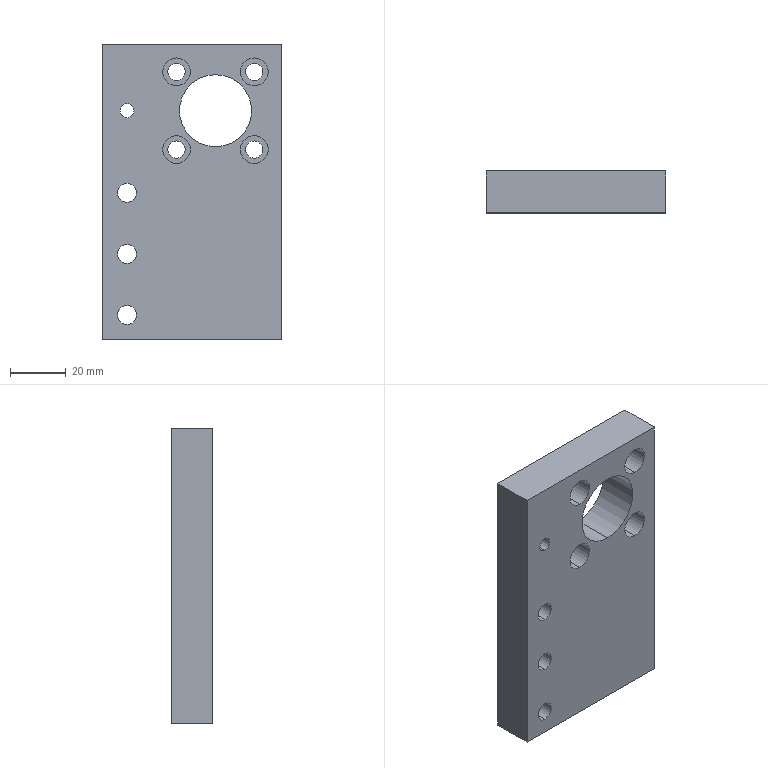Part | 1 solid | 45 faces | box 64.85 x 15 x 106.59 mm | volume 89025 mm3 | cylinder 32 | plane 13 | commonest cylinder face diameters 6.2 x8 10 x8 6.8 x6 11 x6 5 x2 26 x2
STEP:
#1=CARTESIAN_POINT('',(-23.425,0.,26.795));
#2=VERTEX_POINT('',#1);
#3=CARTESIAN_POINT('',(-23.425,0.,31.795));
#4=VERTEX_POINT('',#3);
#5=CARTESIAN_POINT('',(-23.425,0.,29.295));
#6=DIRECTION('',(0.,1.,0.));
#7=DIRECTION('',(0.,0.,1.));
#8=AXIS2_PLACEMENT_3D('',#5,#6,#7);
#9=CIRCLE('',#8,2.5);
#10=EDGE_CURVE('',#2,#4,#9,.T.);
#11=ORIENTED_EDGE('',*,*,#10,.F.);
#12=CARTESIAN_POINT('',(-23.425,15.,26.795));
#13=VERTEX_POINT('',#12);
#14=CARTESIAN_POINT('',(-23.425,15.,26.795));
#15=DIRECTION('',(0.,1.,0.));
#16=VECTOR('',#15,1000.);
#17=LINE('',#14,#16);
#18=EDGE_CURVE('',#2,#13,#17,.T.);
#19=ORIENTED_EDGE('',*,*,#18,.T.);
#20=CARTESIAN_POINT('',(-23.425,15.,31.795));
#21=VERTEX_POINT('',#20);
#22=CARTESIAN_POINT('',(-23.425,15.,29.295));
#23=DIRECTION('',(0.,1.,0.));
#24=DIRECTION('',(0.,0.,1.));
#25=AXIS2_PLACEMENT_3D('',#22,#23,#24);
#26=CIRCLE('',#25,2.5);
#27=EDGE_CURVE('',#13,#21,#26,.T.);
#28=ORIENTED_EDGE('',*,*,#27,.T.);
#29=CARTESIAN_POINT('',(-23.425,15.,31.795));
#30=DIRECTION('',(0.,1.,0.));
#31=VECTOR('',#30,1000.);
#32=LINE('',#29,#31);
#33=EDGE_CURVE('',#4,#21,#32,.T.);
#34=ORIENTED_EDGE('',*,*,#33,.F.);
#35=EDGE_LOOP('',(#11,#19,#28,#34));
#36=FACE_OUTER_BOUND('',#35,.T.);
#37=CARTESIAN_POINT('',(-23.425,15.,29.295));
#38=DIRECTION('',(0.,1.,0.));
#39=DIRECTION('',(0.,0.,1.));
#40=AXIS2_PLACEMENT_3D('',#37,#38,#39);
#41=CYLINDRICAL_SURFACE('',#40,2.5);
#42=ADVANCED_FACE('',(#36),#41,.F.);
#43=CARTESIAN_POINT('',(22.425,8.,48.295));
#44=VERTEX_POINT('',#43);
#45=CARTESIAN_POINT('',(22.425,8.,38.295));
#46=VERTEX_POINT('',#45);
#47=CARTESIAN_POINT('',(22.425,8.,43.295));
#48=DIRECTION('',(0.,-1.,0.));
#49=DIRECTION('',(0.,0.,-1.));
#50=AXIS2_PLACEMENT_3D('',#47,#48,#49);
#51=CIRCLE('',#50,5.);
#52=EDGE_CURVE('',#44,#46,#51,.T.);
#53=ORIENTED_EDGE('',*,*,#52,.F.);
#54=CARTESIAN_POINT('',(22.425,0.,48.295));
#55=VERTEX_POINT('',#54);
#56=CARTESIAN_POINT('',(22.425,8.,48.295));
#57=DIRECTION('',(0.,-1.,0.));
#58=VECTOR('',#57,1000.);
#59=LINE('',#56,#58);
#60=EDGE_CURVE('',#44,#55,#59,.T.);
#61=ORIENTED_EDGE('',*,*,#60,.T.);
#62=CARTESIAN_POINT('',(22.425,0.,38.295));
#63=VERTEX_POINT('',#62);
#64=CARTESIAN_POINT('',(22.425,0.,43.295));
#65=DIRECTION('',(0.,-1.,0.));
#66=DIRECTION('',(0.,0.,-1.));
#67=AXIS2_PLACEMENT_3D('',#64,#65,#66);
#68=CIRCLE('',#67,5.);
#69=EDGE_CURVE('',#55,#63,#68,.T.);
#70=ORIENTED_EDGE('',*,*,#69,.T.);
#71=CARTESIAN_POINT('',(22.425,8.,38.295));
#72=DIRECTION('',(0.,-1.,0.));
#73=VECTOR('',#72,1000.);
#74=LINE('',#71,#73);
#75=EDGE_CURVE('',#46,#63,#74,.T.);
#76=ORIENTED_EDGE('',*,*,#75,.F.);
#77=EDGE_LOOP('',(#53,#61,#70,#76));
#78=FACE_OUTER_BOUND('',#77,.T.);
#79=CARTESIAN_POINT('',(22.425,8.,43.295));
#80=DIRECTION('',(0.,-1.,0.));
#81=DIRECTION('',(0.,0.,-1.));
#82=AXIS2_PLACEMENT_3D('',#79,#80,#81);
#83=CYLINDRICAL_SURFACE('',#82,5.);
#84=ADVANCED_FACE('',(#78),#83,.F.);
#85=CARTESIAN_POINT('',(-5.575,8.,48.295));
#86=VERTEX_POINT('',#85);
#87=CARTESIAN_POINT('',(-5.575,8.,38.295));
#88=VERTEX_POINT('',#87);
#89=CARTESIAN_POINT('',(-5.575,8.,43.295));
#90=DIRECTION('',(0.,-1.,0.));
#91=DIRECTION('',(0.,0.,-1.));
#92=AXIS2_PLACEMENT_3D('',#89,#90,#91);
#93=CIRCLE('',#92,5.);
#94=EDGE_CURVE('',#86,#88,#93,.T.);
#95=ORIENTED_EDGE('',*,*,#94,.F.);
#96=CARTESIAN_POINT('',(-5.575,0.,48.295));
#97=VERTEX_POINT('',#96);
#98=CARTESIAN_POINT('',(-5.575,8.,48.295));
#99=DIRECTION('',(0.,-1.,0.));
#100=VECTOR('',#99,1000.);
#101=LINE('',#98,#100);
#102=EDGE_CURVE('',#86,#97,#101,.T.);
#103=ORIENTED_EDGE('',*,*,#102,.T.);
#104=CARTESIAN_POINT('',(-5.575,0.,38.295));
#105=VERTEX_POINT('',#104);
#106=CARTESIAN_POINT('',(-5.575,0.,43.295));
#107=DIRECTION('',(0.,-1.,0.));
#108=DIRECTION('',(0.,0.,-1.));
#109=AXIS2_PLACEMENT_3D('',#106,#107,#108);
#110=CIRCLE('',#109,5.);
#111=EDGE_CURVE('',#97,#105,#110,.T.);
#112=ORIENTED_EDGE('',*,*,#111,.T.);
#113=CARTESIAN_POINT('',(-5.575,8.,38.295));
#114=DIRECTION('',(0.,-1.,0.));
#115=VECTOR('',#114,1000.);
#116=LINE('',#113,#115);
#117=EDGE_CURVE('',#88,#105,#116,.T.);
#118=ORIENTED_EDGE('',*,*,#117,.F.);
#119=EDGE_LOOP('',(#95,#103,#112,#118));
#120=FACE_OUTER_BOUND('',#119,.T.);
#121=CARTESIAN_POINT('',(-5.575,8.,43.295));
#122=DIRECTION('',(0.,-1.,0.));
#123=DIRECTION('',(0.,0.,-1.));
#124=AXIS2_PLACEMENT_3D('',#121,#122,#123);
#125=CYLINDRICAL_SURFACE('',#124,5.);
#126=ADVANCED_FACE('',(#120),#125,.F.);
#127=CARTESIAN_POINT('',(-5.575,8.,20.295));
#128=VERTEX_POINT('',#127);
#129=CARTESIAN_POINT('',(-5.575,8.,10.295));
#130=VERTEX_POINT('',#129);
#131=CARTESIAN_POINT('',(-5.575,8.,15.295));
#132=DIRECTION('',(0.,-1.,0.));
#133=DIRECTION('',(0.,0.,-1.));
#134=AXIS2_PLACEMENT_3D('',#131,#132,#133);
#135=CIRCLE('',#134,5.);
#136=EDGE_CURVE('',#128,#130,#135,.T.);
#137=ORIENTED_EDGE('',*,*,#136,.F.);
#138=CARTESIAN_POINT('',(-5.575,0.,20.295));
#139=VERTEX_POINT('',#138);
#140=CARTESIAN_POINT('',(-5.575,8.,20.295));
#141=DIRECTION('',(0.,-1.,0.));
#142=VECTOR('',#141,1000.);
#143=LINE('',#140,#142);
#144=EDGE_CURVE('',#128,#139,#143,.T.);
#145=ORIENTED_EDGE('',*,*,#144,.T.);
#146=CARTESIAN_POINT('',(-5.575,0.,10.295));
#147=VERTEX_POINT('',#146);
#148=CARTESIAN_POINT('',(-5.575,0.,15.295));
#149=DIRECTION('',(0.,-1.,0.));
#150=DIRECTION('',(0.,0.,-1.));
#151=AXIS2_PLACEMENT_3D('',#148,#149,#150);
#152=CIRCLE('',#151,5.);
#153=EDGE_CURVE('',#139,#147,#152,.T.);
#154=ORIENTED_EDGE('',*,*,#153,.T.);
#155=CARTESIAN_POINT('',(-5.575,8.,10.295));
#156=DIRECTION('',(0.,-1.,0.));
#157=VECTOR('',#156,1000.);
#158=LINE('',#155,#157);
#159=EDGE_CURVE('',#130,#147,#158,.T.);
#160=ORIENTED_EDGE('',*,*,#159,.F.);
#161=EDGE_LOOP('',(#137,#145,#154,#160));
#162=FACE_OUTER_BOUND('',#161,.T.);
#163=CARTESIAN_POINT('',(-5.575,8.,15.295));
#164=DIRECTION('',(0.,-1.,0.));
#165=DIRECTION('',(0.,0.,-1.));
#166=AXIS2_PLACEMENT_3D('',#163,#164,#165);
#167=CYLINDRICAL_SURFACE('',#166,5.);
#168=ADVANCED_FACE('',(#162),#167,.F.);
#169=CARTESIAN_POINT('',(22.425,8.,20.295));
#170=VERTEX_POINT('',#169);
#171=CARTESIAN_POINT('',(22.425,8.,10.295));
#172=VERTEX_POINT('',#171);
#173=CARTESIAN_POINT('',(22.425,8.,15.295));
#174=DIRECTION('',(0.,-1.,0.));
#175=DIRECTION('',(0.,0.,-1.));
#176=AXIS2_PLACEMENT_3D('',#173,#174,#175);
#177=CIRCLE('',#176,5.);
#178=EDGE_CURVE('',#170,#172,#177,.T.);
#179=ORIENTED_EDGE('',*,*,#178,.F.);
#180=CARTESIAN_POINT('',(22.425,0.,20.295));
#181=VERTEX_POINT('',#180);
#182=CARTESIAN_POINT('',(22.425,8.,20.295));
#183=DIRECTION('',(0.,-1.,0.));
#184=VECTOR('',#183,1000.);
#185=LINE('',#182,#184);
#186=EDGE_CURVE('',#170,#181,#185,.T.);
#187=ORIENTED_EDGE('',*,*,#186,.T.);
#188=CARTESIAN_POINT('',(22.425,0.,10.295));
#189=VERTEX_POINT('',#188);
#190=CARTESIAN_POINT('',(22.425,0.,15.295));
#191=DIRECTION('',(0.,-1.,0.));
#192=DIRECTION('',(0.,0.,-1.));
#193=AXIS2_PLACEMENT_3D('',#190,#191,#192);
#194=CIRCLE('',#193,5.);
#195=EDGE_CURVE('',#181,#189,#194,.T.);
#196=ORIENTED_EDGE('',*,*,#195,.T.);
#197=CARTESIAN_POINT('',(22.425,8.,10.295));
#198=DIRECTION('',(0.,-1.,0.));
#199=VECTOR('',#198,1000.);
#200=LINE('',#197,#199);
#201=EDGE_CURVE('',#172,#189,#200,.T.);
#202=ORIENTED_EDGE('',*,*,#201,.F.);
#203=EDGE_LOOP('',(#179,#187,#196,#202));
#204=FACE_OUTER_BOUND('',#203,.T.);
#205=CARTESIAN_POINT('',(22.425,8.,15.295));
#206=DIRECTION('',(0.,-1.,0.));
#207=DIRECTION('',(0.,0.,-1.));
#208=AXIS2_PLACEMENT_3D('',#205,#206,#207);
#209=CYLINDRICAL_SURFACE('',#208,5.);
#210=ADVANCED_FACE('',(#204),#209,.F.);
#211=CARTESIAN_POINT('',(8.475,0.,16.295));
#212=VERTEX_POINT('',#211);
#213=CARTESIAN_POINT('',(8.475,0.,42.295));
#214=VERTEX_POINT('',#213);
#215=CARTESIAN_POINT('',(8.475,0.,29.295));
#216=DIRECTION('',(0.,1.,0.));
#217=DIRECTION('',(0.,0.,1.));
#218=AXIS2_PLACEMENT_3D('',#215,#216,#217);
#219=CIRCLE('',#218,13.);
#220=EDGE_CURVE('',#212,#214,#219,.T.);
#221=ORIENTED_EDGE('',*,*,#220,.F.);
#222=CARTESIAN_POINT('',(8.475,15.,16.295));
#223=VERTEX_POINT('',#222);
#224=CARTESIAN_POINT('',(8.475,0.,16.295));
#225=DIRECTION('',(0.,1.,0.));
#226=VECTOR('',#225,1000.);
#227=LINE('',#224,#226);
#228=EDGE_CURVE('',#212,#223,#227,.T.);
#229=ORIENTED_EDGE('',*,*,#228,.T.);
#230=CARTESIAN_POINT('',(8.475,15.,42.295));
#231=VERTEX_POINT('',#230);
#232=CARTESIAN_POINT('',(8.475,15.,29.295));
#233=DIRECTION('',(0.,1.,0.));
#234=DIRECTION('',(0.,0.,1.));
#235=AXIS2_PLACEMENT_3D('',#232,#233,#234);
#236=CIRCLE('',#235,13.);
#237=EDGE_CURVE('',#223,#231,#236,.T.);
#238=ORIENTED_EDGE('',*,*,#237,.T.);
#239=CARTESIAN_POINT('',(8.475,0.,42.295));
#240=DIRECTION('',(0.,1.,0.));
#241=VECTOR('',#240,1000.);
#242=LINE('',#239,#241);
#243=EDGE_CURVE('',#214,#231,#242,.T.);
#244=ORIENTED_EDGE('',*,*,#243,.F.);
#245=EDGE_LOOP('',(#221,#229,#238,#244));
#246=FACE_OUTER_BOUND('',#245,.T.);
#247=CARTESIAN_POINT('',(8.475,0.,29.295));
#248=DIRECTION('',(0.,1.,0.));
#249=DIRECTION('',(0.,0.,1.));
#250=AXIS2_PLACEMENT_3D('',#247,#248,#249);
#251=CYLINDRICAL_SURFACE('',#250,13.);
#252=ADVANCED_FACE('',(#246),#251,.F.);
#253=CARTESIAN_POINT('',(-23.425,7.,-5.795));
#254=VERTEX_POINT('',#253);
#255=CARTESIAN_POINT('',(-23.425,7.,5.205));
#256=VERTEX_POINT('',#255);
#257=CARTESIAN_POINT('',(-23.425,7.,-0.295));
#258=DIRECTION('',(0.,1.,0.));
#259=DIRECTION('',(0.,0.,1.));
#260=AXIS2_PLACEMENT_3D('',#257,#258,#259);
#261=CIRCLE('',#260,5.5);
#262=EDGE_CURVE('',#254,#256,#261,.T.);
#263=ORIENTED_EDGE('',*,*,#262,.F.);
#264=CARTESIAN_POINT('',(-23.425,15.,-5.795));
#265=VERTEX_POINT('',#264);
#266=CARTESIAN_POINT('',(-23.425,7.,-5.795));
#267=DIRECTION('',(0.,1.,0.));
#268=VECTOR('',#267,1000.);
#269=LINE('',#266,#268);
#270=EDGE_CURVE('',#254,#265,#269,.T.);
#271=ORIENTED_EDGE('',*,*,#270,.T.);
#272=CARTESIAN_POINT('',(-23.425,15.,5.205));
#273=VERTEX_POINT('',#272);
#274=CARTESIAN_POINT('',(-23.425,15.,-0.295));
#275=DIRECTION('',(0.,1.,0.));
#276=DIRECTION('',(0.,0.,1.));
#277=AXIS2_PLACEMENT_3D('',#274,#275,#276);
#278=CIRCLE('',#277,5.5);
#279=EDGE_CURVE('',#265,#273,#278,.T.);
#280=ORIENTED_EDGE('',*,*,#279,.T.);
#281=CARTESIAN_POINT('',(-23.425,7.,5.205));
#282=DIRECTION('',(0.,1.,0.));
#283=VECTOR('',#282,1000.);
#284=LINE('',#281,#283);
#285=EDGE_CURVE('',#256,#273,#284,.T.);
#286=ORIENTED_EDGE('',*,*,#285,.F.);
#287=EDGE_LOOP('',(#263,#271,#280,#286));
#288=FACE_OUTER_BOUND('',#287,.T.);
#289=CARTESIAN_POINT('',(-23.425,7.,-0.295));
#290=DIRECTION('',(0.,1.,0.));
#291=DIRECTION('',(0.,0.,1.));
#292=AXIS2_PLACEMENT_3D('',#289,#290,#291);
#293=CYLINDRICAL_SURFACE('',#292,5.5);
#294=ADVANCED_FACE('',(#288),#293,.F.);
#295=CARTESIAN_POINT('',(-23.425,7.,-27.795));
#296=VERTEX_POINT('',#295);
#297=CARTESIAN_POINT('',(-23.425,7.,-16.795));
#298=VERTEX_POINT('',#297);
#299=CARTESIAN_POINT('',(-23.425,7.,-22.295));
#300=DIRECTION('',(0.,1.,0.));
#301=DIRECTION('',(0.,0.,1.));
#302=AXIS2_PLACEMENT_3D('',#299,#300,#301);
#303=CIRCLE('',#302,5.5);
#304=EDGE_CURVE('',#296,#298,#303,.T.);
#305=ORIENTED_EDGE('',*,*,#304,.F.);
#306=CARTESIAN_POINT('',(-23.425,15.,-27.795));
#307=VERTEX_POINT('',#306);
#308=CARTESIAN_POINT('',(-23.425,7.,-27.795));
#309=DIRECTION('',(0.,1.,0.));
#310=VECTOR('',#309,1000.);
#311=LINE('',#308,#310);
#312=EDGE_CURVE('',#296,#307,#311,.T.);
#313=ORIENTED_EDGE('',*,*,#312,.T.);
#314=CARTESIAN_POINT('',(-23.425,15.,-16.795));
#315=VERTEX_POINT('',#314);
#316=CARTESIAN_POINT('',(-23.425,15.,-22.295));
#317=DIRECTION('',(0.,1.,0.));
#318=DIRECTION('',(0.,0.,1.));
#319=AXIS2_PLACEMENT_3D('',#316,#317,#318);
#320=CIRCLE('',#319,5.5);
#321=EDGE_CURVE('',#307,#315,#320,.T.);
#322=ORIENTED_EDGE('',*,*,#321,.T.);
#323=CARTESIAN_POINT('',(-23.425,7.,-16.795));
#324=DIRECTION('',(0.,1.,0.));
#325=VECTOR('',#324,1000.);
#326=LINE('',#323,#325);
#327=EDGE_CURVE('',#298,#315,#326,.T.);
#328=ORIENTED_EDGE('',*,*,#327,.F.);
#329=EDGE_LOOP('',(#305,#313,#322,#328));
#330=FACE_OUTER_BOUND('',#329,.T.);
#331=CARTESIAN_POINT('',(-23.425,7.,-22.295));
#332=DIRECTION('',(0.,1.,0.));
#333=DIRECTION('',(0.,0.,1.));
#334=AXIS2_PLACEMENT_3D('',#331,#332,#333);
#335=CYLINDRICAL_SURFACE('',#334,5.5);
#336=ADVANCED_FACE('',(#330),#335,.F.);
#337=CARTESIAN_POINT('',(-23.425,7.,-49.795));
#338=VERTEX_POINT('',#337);
#339=CARTESIAN_POINT('',(-23.425,7.,-38.795));
#340=VERTEX_POINT('',#339);
#341=CARTESIAN_POINT('',(-23.425,7.,-44.295));
#342=DIRECTION('',(0.,1.,0.));
#343=DIRECTION('',(0.,0.,1.));
#344=AXIS2_PLACEMENT_3D('',#341,#342,#343);
#345=CIRCLE('',#344,5.5);
#346=EDGE_CURVE('',#338,#340,#345,.T.);
#347=ORIENTED_EDGE('',*,*,#346,.F.);
#348=CARTESIAN_POINT('',(-23.425,15.,-49.795));
#349=VERTEX_POINT('',#348);
#350=CARTESIAN_POINT('',(-23.425,7.,-49.795));
#351=DIRECTION('',(0.,1.,0.));
#352=VECTOR('',#351,1000.);
#353=LINE('',#350,#352);
#354=EDGE_CURVE('',#338,#349,#353,.T.);
#355=ORIENTED_EDGE('',*,*,#354,.T.);
#356=CARTESIAN_POINT('',(-23.425,15.,-38.795));
#357=VERTEX_POINT('',#356);
#358=CARTESIAN_POINT('',(-23.425,15.,-44.295));
#359=DIRECTION('',(0.,1.,0.));
#360=DIRECTION('',(0.,0.,1.));
#361=AXIS2_PLACEMENT_3D('',#358,#359,#360);
#362=CIRCLE('',#361,5.5);
#363=EDGE_CURVE('',#349,#357,#362,.T.);
#364=ORIENTED_EDGE('',*,*,#363,.T.);
#365=CARTESIAN_POINT('',(-23.425,7.,-38.795));
#366=DIRECTION('',(0.,1.,0.));
#367=VECTOR('',#366,1000.);
#368=LINE('',#365,#367);
#369=EDGE_CURVE('',#340,#357,#368,.T.);
#370=ORIENTED_EDGE('',*,*,#369,.F.);
#371=EDGE_LOOP('',(#347,#355,#364,#370));
#372=FACE_OUTER_BOUND('',#371,.T.);
#373=CARTESIAN_POINT('',(-23.425,7.,-44.295));
#374=DIRECTION('',(0.,1.,0.));
#375=DIRECTION('',(0.,0.,1.));
#376=AXIS2_PLACEMENT_3D('',#373,#374,#375);
#377=CYLINDRICAL_SURFACE('',#376,5.5);
#378=ADVANCED_FACE('',(#372),#377,.F.);
#379=CARTESIAN_POINT('',(-23.425,0.,-47.695));
#380=VERTEX_POINT('',#379);
#381=CARTESIAN_POINT('',(-23.425,0.,-40.895));
#382=VERTEX_POINT('',#381);
#383=CARTESIAN_POINT('',(-23.425,0.,-44.295));
#384=DIRECTION('',(0.,1.,0.));
#385=DIRECTION('',(0.,0.,1.));
#386=AXIS2_PLACEMENT_3D('',#383,#384,#385);
#387=CIRCLE('',#386,3.4);
#388=EDGE_CURVE('',#380,#382,#387,.T.);
#389=ORIENTED_EDGE('',*,*,#388,.F.);
#390=CARTESIAN_POINT('',(-23.425,7.,-47.695));
#391=VERTEX_POINT('',#390);
#392=CARTESIAN_POINT('',(-23.425,0.,-47.695));
#393=DIRECTION('',(0.,1.,0.));
#394=VECTOR('',#393,1000.);
#395=LINE('',#392,#394);
#396=EDGE_CURVE('',#380,#391,#395,.T.);
#397=ORIENTED_EDGE('',*,*,#396,.T.);
#398=CARTESIAN_POINT('',(-23.425,7.,-40.895));
#399=VERTEX_POINT('',#398);
#400=CARTESIAN_POINT('',(-23.425,7.,-44.295));
#401=DIRECTION('',(0.,-1.,0.));
#402=DIRECTION('',(0.,0.,1.));
#403=AXIS2_PLACEMENT_3D('',#400,#401,#402);
#404=CIRCLE('',#403,3.4);
#405=EDGE_CURVE('',#399,#391,#404,.T.);
#406=ORIENTED_EDGE('',*,*,#405,.F.);
#407=CARTESIAN_POINT('',(-23.425,0.,-40.895));
#408=DIRECTION('',(0.,1.,0.));
#409=VECTOR('',#408,1000.);
#410=LINE('',#407,#409);
#411=EDGE_CURVE('',#382,#399,#410,.T.);
#412=ORIENTED_EDGE('',*,*,#411,.F.);
#413=EDGE_LOOP('',(#389,#397,#406,#412));
#414=FACE_OUTER_BOUND('',#413,.T.);
#415=CARTESIAN_POINT('',(-23.425,0.,-44.295));
#416=DIRECTION('',(0.,1.,0.));
#417=DIRECTION('',(0.,0.,1.));
#418=AXIS2_PLACEMENT_3D('',#415,#416,#417);
#419=CYLINDRICAL_SURFACE('',#418,3.4);
#420=ADVANCED_FACE('',(#414),#419,.F.);
#421=CARTESIAN_POINT('',(-23.425,0.,-25.695));
#422=VERTEX_POINT('',#421);
#423=CARTESIAN_POINT('',(-23.425,0.,-18.895));
#424=VERTEX_POINT('',#423);
#425=CARTESIAN_POINT('',(-23.425,0.,-22.295));
#426=DIRECTION('',(0.,1.,0.));
#427=DIRECTION('',(0.,0.,1.));
#428=AXIS2_PLACEMENT_3D('',#425,#426,#427);
#429=CIRCLE('',#428,3.4);
#430=EDGE_CURVE('',#422,#424,#429,.T.);
#431=ORIENTED_EDGE('',*,*,#430,.F.);
#432=CARTESIAN_POINT('',(-23.425,7.,-25.695));
#433=VERTEX_POINT('',#432);
#434=CARTESIAN_POINT('',(-23.425,0.,-25.695));
#435=DIRECTION('',(0.,1.,0.));
#436=VECTOR('',#435,1000.);
#437=LINE('',#434,#436);
#438=EDGE_CURVE('',#422,#433,#437,.T.);
#439=ORIENTED_EDGE('',*,*,#438,.T.);
#440=CARTESIAN_POINT('',(-23.425,7.,-18.895));
#441=VERTEX_POINT('',#440);
#442=CARTESIAN_POINT('',(-23.425,7.,-22.295));
#443=DIRECTION('',(0.,-1.,0.));
#444=DIRECTION('',(0.,0.,1.));
#445=AXIS2_PLACEMENT_3D('',#442,#443,#444);
#446=CIRCLE('',#445,3.4);
#447=EDGE_CURVE('',#441,#433,#446,.T.);
#448=ORIENTED_EDGE('',*,*,#447,.F.);
#449=CARTESIAN_POINT('',(-23.425,0.,-18.895));
#450=DIRECTION('',(0.,1.,0.));
#451=VECTOR('',#450,1000.);
#452=LINE('',#449,#451);
#453=EDGE_CURVE('',#424,#441,#452,.T.);
#454=ORIENTED_EDGE('',*,*,#453,.F.);
#455=EDGE_LOOP('',(#431,#439,#448,#454));
#456=FACE_OUTER_BOUND('',#455,.T.);
#457=CARTESIAN_POINT('',(-23.425,0.,-22.295));
#458=DIRECTION('',(0.,1.,0.));
#459=DIRECTION('',(0.,0.,1.));
#460=AXIS2_PLACEMENT_3D('',#457,#458,#459);
#461=CYLINDRICAL_SURFACE('',#460,3.4);
#462=ADVANCED_FACE('',(#456),#461,.F.);
#463=CARTESIAN_POINT('',(-23.425,0.,-3.695));
#464=VERTEX_POINT('',#463);
#465=CARTESIAN_POINT('',(-23.425,0.,3.105));
#466=VERTEX_POINT('',#465);
#467=CARTESIAN_POINT('',(-23.425,0.,-0.295));
#468=DIRECTION('',(0.,1.,0.));
#469=DIRECTION('',(0.,0.,1.));
#470=AXIS2_PLACEMENT_3D('',#467,#468,#469);
#471=CIRCLE('',#470,3.4);
#472=EDGE_CURVE('',#464,#466,#471,.T.);
#473=ORIENTED_EDGE('',*,*,#472,.F.);
#474=CARTESIAN_POINT('',(-23.425,7.,-3.695));
#475=VERTEX_POINT('',#474);
#476=CARTESIAN_POINT('',(-23.425,0.,-3.695));
#477=DIRECTION('',(0.,1.,0.));
#478=VECTOR('',#477,1000.);
#479=LINE('',#476,#478);
#480=EDGE_CURVE('',#464,#475,#479,.T.);
#481=ORIENTED_EDGE('',*,*,#480,.T.);
#482=CARTESIAN_POINT('',(-23.425,7.,3.105));
#483=VERTEX_POINT('',#482);
#484=CARTESIAN_POINT('',(-23.425,7.,-0.295));
#485=DIRECTION('',(0.,-1.,0.));
#486=DIRECTION('',(0.,0.,1.));
#487=AXIS2_PLACEMENT_3D('',#484,#485,#486);
#488=CIRCLE('',#487,3.4);
#489=EDGE_CURVE('',#483,#475,#488,.T.);
#490=ORIENTED_EDGE('',*,*,#489,.F.);
#491=CARTESIAN_POINT('',(-23.425,0.,3.105));
#492=DIRECTION('',(0.,1.,0.));
#493=VECTOR('',#492,1000.);
#494=LINE('',#491,#493);
#495=EDGE_CURVE('',#466,#483,#494,.T.);
#496=ORIENTED_EDGE('',*,*,#495,.F.);
#497=EDGE_LOOP('',(#473,#481,#490,#496));
#498=FACE_OUTER_BOUND('',#497,.T.);
#499=CARTESIAN_POINT('',(-23.425,0.,-0.295));
#500=DIRECTION('',(0.,1.,0.));
#501=DIRECTION('',(0.,0.,1.));
#502=AXIS2_PLACEMENT_3D('',#499,#500,#501);
#503=CYLINDRICAL_SURFACE('',#502,3.4);
#504=ADVANCED_FACE('',(#498),#503,.F.);
#505=CARTESIAN_POINT('',(22.425,8.,12.195));
#506=VERTEX_POINT('',#505);
#507=CARTESIAN_POINT('',(22.425,8.,18.395));
#508=VERTEX_POINT('',#507);
#509=CARTESIAN_POINT('',(22.425,8.,15.295));
#510=DIRECTION('',(0.,1.,0.));
#511=DIRECTION('',(0.,0.,-1.));
#512=AXIS2_PLACEMENT_3D('',#509,#510,#511);
#513=CIRCLE('',#512,3.1);
#514=EDGE_CURVE('',#506,#508,#513,.T.);
#515=ORIENTED_EDGE('',*,*,#514,.F.);
#516=CARTESIAN_POINT('',(22.425,15.,12.195));
#517=VERTEX_POINT('',#516);
#518=CARTESIAN_POINT('',(22.425,0.,12.195));
#519=DIRECTION('',(0.,1.,0.));
#520=VECTOR('',#519,1000.);
#521=LINE('',#518,#520);
#522=EDGE_CURVE('',#506,#517,#521,.T.);
#523=ORIENTED_EDGE('',*,*,#522,.T.);
#524=CARTESIAN_POINT('',(22.425,15.,18.395));
#525=VERTEX_POINT('',#524);
#526=CARTESIAN_POINT('',(22.425,15.,15.295));
#527=DIRECTION('',(0.,1.,0.));
#528=DIRECTION('',(0.,0.,1.));
#529=AXIS2_PLACEMENT_3D('',#526,#527,#528);
#530=CIRCLE('',#529,3.1);
#531=EDGE_CURVE('',#517,#525,#530,.T.);
#532=ORIENTED_EDGE('',*,*,#531,.T.);
#533=CARTESIAN_POINT('',(22.425,0.,18.395));
#534=DIRECTION('',(0.,1.,0.));
#535=VECTOR('',#534,1000.);
#536=LINE('',#533,#535);
#537=EDGE_CURVE('',#508,#525,#536,.T.);
#538=ORIENTED_EDGE('',*,*,#537,.F.);
#539=EDGE_LOOP('',(#515,#523,#532,#538));
#540=FACE_OUTER_BOUND('',#539,.T.);
#541=CARTESIAN_POINT('',(22.425,0.,15.295));
#542=DIRECTION('',(0.,1.,0.));
#543=DIRECTION('',(0.,0.,1.));
#544=AXIS2_PLACEMENT_3D('',#541,#542,#543);
#545=CYLINDRICAL_SURFACE('',#544,3.1);
#546=ADVANCED_FACE('',(#540),#545,.F.);
#547=CARTESIAN_POINT('',(-5.575,8.,12.195));
#548=VERTEX_POINT('',#547);
#549=CARTESIAN_POINT('',(-5.575,8.,18.395));
#550=VERTEX_POINT('',#549);
#551=CARTESIAN_POINT('',(-5.575,8.,15.295));
#552=DIRECTION('',(0.,1.,0.));
#553=DIRECTION('',(0.,0.,-1.));
#554=AXIS2_PLACEMENT_3D('',#551,#552,#553);
#555=CIRCLE('',#554,3.1);
#556=EDGE_CURVE('',#548,#550,#555,.T.);
#557=ORIENTED_EDGE('',*,*,#556,.F.);
#558=CARTESIAN_POINT('',(-5.575,15.,12.195));
#559=VERTEX_POINT('',#558);
#560=CARTESIAN_POINT('',(-5.575,0.,12.195));
#561=DIRECTION('',(0.,1.,0.));
#562=VECTOR('',#561,1000.);
#563=LINE('',#560,#562);
#564=EDGE_CURVE('',#548,#559,#563,.T.);
#565=ORIENTED_EDGE('',*,*,#564,.T.);
#566=CARTESIAN_POINT('',(-5.575,15.,18.395));
#567=VERTEX_POINT('',#566);
#568=CARTESIAN_POINT('',(-5.575,15.,15.295));
#569=DIRECTION('',(0.,1.,0.));
#570=DIRECTION('',(0.,0.,1.));
#571=AXIS2_PLACEMENT_3D('',#568,#569,#570);
#572=CIRCLE('',#571,3.1);
#573=EDGE_CURVE('',#559,#567,#572,.T.);
#574=ORIENTED_EDGE('',*,*,#573,.T.);
#575=CARTESIAN_POINT('',(-5.575,0.,18.395));
#576=DIRECTION('',(0.,1.,0.));
#577=VECTOR('',#576,1000.);
#578=LINE('',#575,#577);
#579=EDGE_CURVE('',#550,#567,#578,.T.);
#580=ORIENTED_EDGE('',*,*,#579,.F.);
#581=EDGE_LOOP('',(#557,#565,#574,#580));
#582=FACE_OUTER_BOUND('',#581,.T.);
#583=CARTESIAN_POINT('',(-5.575,0.,15.295));
#584=DIRECTION('',(0.,1.,0.));
#585=DIRECTION('',(0.,0.,1.));
#586=AXIS2_PLACEMENT_3D('',#583,#584,#585);
#587=CYLINDRICAL_SURFACE('',#586,3.1);
#588=ADVANCED_FACE('',(#582),#587,.F.);
#589=CARTESIAN_POINT('',(-5.575,8.,40.195));
#590=VERTEX_POINT('',#589);
#591=CARTESIAN_POINT('',(-5.575,8.,46.395));
#592=VERTEX_POINT('',#591);
#593=CARTESIAN_POINT('',(-5.575,8.,43.295));
#594=DIRECTION('',(0.,1.,0.));
#595=DIRECTION('',(0.,0.,-1.));
#596=AXIS2_PLACEMENT_3D('',#593,#594,#595);
#597=CIRCLE('',#596,3.1);
#598=EDGE_CURVE('',#590,#592,#597,.T.);
#599=ORIENTED_EDGE('',*,*,#598,.F.);
#600=CARTESIAN_POINT('',(-5.575,15.,40.195));
#601=VERTEX_POINT('',#600);
#602=CARTESIAN_POINT('',(-5.575,0.,40.195));
#603=DIRECTION('',(0.,1.,0.));
#604=VECTOR('',#603,1000.);
#605=LINE('',#602,#604);
#606=EDGE_CURVE('',#590,#601,#605,.T.);
#607=ORIENTED_EDGE('',*,*,#606,.T.);
#608=CARTESIAN_POINT('',(-5.575,15.,46.395));
#609=VERTEX_POINT('',#608);
#610=CARTESIAN_POINT('',(-5.575,15.,43.295));
#611=DIRECTION('',(0.,1.,0.));
#612=DIRECTION('',(0.,0.,1.));
#613=AXIS2_PLACEMENT_3D('',#610,#611,#612);
#614=CIRCLE('',#613,3.1);
#615=EDGE_CURVE('',#601,#609,#614,.T.);
#616=ORIENTED_EDGE('',*,*,#615,.T.);
#617=CARTESIAN_POINT('',(-5.575,0.,46.395));
#618=DIRECTION('',(0.,1.,0.));
#619=VECTOR('',#618,1000.);
#620=LINE('',#617,#619);
#621=EDGE_CURVE('',#592,#609,#620,.T.);
#622=ORIENTED_EDGE('',*,*,#621,.F.);
#623=EDGE_LOOP('',(#599,#607,#616,#622));
#624=FACE_OUTER_BOUND('',#623,.T.);
#625=CARTESIAN_POINT('',(-5.575,0.,43.295));
#626=DIRECTION('',(0.,1.,0.));
#627=DIRECTION('',(0.,0.,1.));
#628=AXIS2_PLACEMENT_3D('',#625,#626,#627);
#629=CYLINDRICAL_SURFACE('',#628,3.1);
#630=ADVANCED_FACE('',(#624),#629,.F.);
#631=CARTESIAN_POINT('',(22.425,8.,40.195));
#632=VERTEX_POINT('',#631);
#633=CARTESIAN_POINT('',(22.425,8.,46.395));
#634=VERTEX_POINT('',#633);
#635=CARTESIAN_POINT('',(22.425,8.,43.295));
#636=DIRECTION('',(0.,1.,0.));
#637=DIRECTION('',(0.,0.,-1.));
#638=AXIS2_PLACEMENT_3D('',#635,#636,#637);
#639=CIRCLE('',#638,3.1);
#640=EDGE_CURVE('',#632,#634,#639,.T.);
#641=ORIENTED_EDGE('',*,*,#640,.F.);
#642=CARTESIAN_POINT('',(22.425,15.,40.195));
#643=VERTEX_POINT('',#642);
#644=CARTESIAN_POINT('',(22.425,0.,40.195));
#645=DIRECTION('',(0.,1.,0.));
#646=VECTOR('',#645,1000.);
#647=LINE('',#644,#646);
#648=EDGE_CURVE('',#632,#643,#647,.T.);
#649=ORIENTED_EDGE('',*,*,#648,.T.);
#650=CARTESIAN_POINT('',(22.425,15.,46.395));
#651=VERTEX_POINT('',#650);
#652=CARTESIAN_POINT('',(22.425,15.,43.295));
#653=DIRECTION('',(0.,1.,0.));
#654=DIRECTION('',(0.,0.,1.));
#655=AXIS2_PLACEMENT_3D('',#652,#653,#654);
#656=CIRCLE('',#655,3.1);
#657=EDGE_CURVE('',#643,#651,#656,.T.);
#658=ORIENTED_EDGE('',*,*,#657,.T.);
#659=CARTESIAN_POINT('',(22.425,0.,46.395));
#660=DIRECTION('',(0.,1.,0.));
#661=VECTOR('',#660,1000.);
#662=LINE('',#659,#661);
#663=EDGE_CURVE('',#634,#651,#662,.T.);
#664=ORIENTED_EDGE('',*,*,#663,.F.);
#665=EDGE_LOOP('',(#641,#649,#658,#664));
#666=FACE_OUTER_BOUND('',#665,.T.);
#667=CARTESIAN_POINT('',(22.425,0.,43.295));
#668=DIRECTION('',(0.,1.,0.));
#669=DIRECTION('',(0.,0.,1.));
#670=AXIS2_PLACEMENT_3D('',#667,#668,#669);
#671=CYLINDRICAL_SURFACE('',#670,3.1);
#672=ADVANCED_FACE('',(#666),#671,.F.);
#673=ORIENTED_EDGE('',*,*,#648,.F.);
#674=CARTESIAN_POINT('',(22.425,8.,43.295));
#675=DIRECTION('',(0.,1.,0.));
#676=DIRECTION('',(0.,0.,-1.));
#677=AXIS2_PLACEMENT_3D('',#674,#675,#676);
#678=CIRCLE('',#677,3.1);
#679=EDGE_CURVE('',#634,#632,#678,.T.);
#680=ORIENTED_EDGE('',*,*,#679,.F.);
#681=ORIENTED_EDGE('',*,*,#663,.T.);
#682=CARTESIAN_POINT('',(22.425,15.,43.295));
#683=DIRECTION('',(0.,1.,0.));
#684=DIRECTION('',(0.,0.,1.));
#685=AXIS2_PLACEMENT_3D('',#682,#683,#684);
#686=CIRCLE('',#685,3.1);
#687=EDGE_CURVE('',#651,#643,#686,.T.);
#688=ORIENTED_EDGE('',*,*,#687,.T.);
#689=EDGE_LOOP('',(#673,#680,#681,#688));
#690=FACE_OUTER_BOUND('',#689,.T.);
#691=CARTESIAN_POINT('',(22.425,0.,43.295));
#692=DIRECTION('',(0.,1.,0.));
#693=DIRECTION('',(0.,0.,1.));
#694=AXIS2_PLACEMENT_3D('',#691,#692,#693);
#695=CYLINDRICAL_SURFACE('',#694,3.1);
#696=ADVANCED_FACE('',(#690),#695,.F.);
#697=ORIENTED_EDGE('',*,*,#606,.F.);
#698=CARTESIAN_POINT('',(-5.575,8.,43.295));
#699=DIRECTION('',(0.,1.,0.));
#700=DIRECTION('',(0.,0.,-1.));
#701=AXIS2_PLACEMENT_3D('',#698,#699,#700);
#702=CIRCLE('',#701,3.1);
#703=EDGE_CURVE('',#592,#590,#702,.T.);
#704=ORIENTED_EDGE('',*,*,#703,.F.);
#705=ORIENTED_EDGE('',*,*,#621,.T.);
#706=CARTESIAN_POINT('',(-5.575,15.,43.295));
#707=DIRECTION('',(0.,1.,0.));
#708=DIRECTION('',(0.,0.,1.));
#709=AXIS2_PLACEMENT_3D('',#706,#707,#708);
#710=CIRCLE('',#709,3.1);
#711=EDGE_CURVE('',#609,#601,#710,.T.);
#712=ORIENTED_EDGE('',*,*,#711,.T.);
#713=EDGE_LOOP('',(#697,#704,#705,#712));
#714=FACE_OUTER_BOUND('',#713,.T.);
#715=CARTESIAN_POINT('',(-5.575,0.,43.295));
#716=DIRECTION('',(0.,1.,0.));
#717=DIRECTION('',(0.,0.,1.));
#718=AXIS2_PLACEMENT_3D('',#715,#716,#717);
#719=CYLINDRICAL_SURFACE('',#718,3.1);
#720=ADVANCED_FACE('',(#714),#719,.F.);
#721=ORIENTED_EDGE('',*,*,#564,.F.);
#722=CARTESIAN_POINT('',(-5.575,8.,15.295));
#723=DIRECTION('',(0.,1.,0.));
#724=DIRECTION('',(0.,0.,-1.));
#725=AXIS2_PLACEMENT_3D('',#722,#723,#724);
#726=CIRCLE('',#725,3.1);
#727=EDGE_CURVE('',#550,#548,#726,.T.);
#728=ORIENTED_EDGE('',*,*,#727,.F.);
#729=ORIENTED_EDGE('',*,*,#579,.T.);
#730=CARTESIAN_POINT('',(-5.575,15.,15.295));
#731=DIRECTION('',(0.,1.,0.));
#732=DIRECTION('',(0.,0.,1.));
#733=AXIS2_PLACEMENT_3D('',#730,#731,#732);
#734=CIRCLE('',#733,3.1);
#735=EDGE_CURVE('',#567,#559,#734,.T.);
#736=ORIENTED_EDGE('',*,*,#735,.T.);
#737=EDGE_LOOP('',(#721,#728,#729,#736));
#738=FACE_OUTER_BOUND('',#737,.T.);
#739=CARTESIAN_POINT('',(-5.575,0.,15.295));
#740=DIRECTION('',(0.,1.,0.));
#741=DIRECTION('',(0.,0.,1.));
#742=AXIS2_PLACEMENT_3D('',#739,#740,#741);
#743=CYLINDRICAL_SURFACE('',#742,3.1);
#744=ADVANCED_FACE('',(#738),#743,.F.);
#745=ORIENTED_EDGE('',*,*,#522,.F.);
#746=CARTESIAN_POINT('',(22.425,8.,15.295));
#747=DIRECTION('',(0.,1.,0.));
#748=DIRECTION('',(0.,0.,-1.));
#749=AXIS2_PLACEMENT_3D('',#746,#747,#748);
#750=CIRCLE('',#749,3.1);
#751=EDGE_CURVE('',#508,#506,#750,.T.);
#752=ORIENTED_EDGE('',*,*,#751,.F.);
#753=ORIENTED_EDGE('',*,*,#537,.T.);
#754=CARTESIAN_POINT('',(22.425,15.,15.295));
#755=DIRECTION('',(0.,1.,0.));
#756=DIRECTION('',(0.,0.,1.));
#757=AXIS2_PLACEMENT_3D('',#754,#755,#756);
#758=CIRCLE('',#757,3.1);
#759=EDGE_CURVE('',#525,#517,#758,.T.);
#760=ORIENTED_EDGE('',*,*,#759,.T.);
#761=EDGE_LOOP('',(#745,#752,#753,#760));
#762=FACE_OUTER_BOUND('',#761,.T.);
#763=CARTESIAN_POINT('',(22.425,0.,15.295));
#764=DIRECTION('',(0.,1.,0.));
#765=DIRECTION('',(0.,0.,1.));
#766=AXIS2_PLACEMENT_3D('',#763,#764,#765);
#767=CYLINDRICAL_SURFACE('',#766,3.1);
#768=ADVANCED_FACE('',(#762),#767,.F.);
#769=ORIENTED_EDGE('',*,*,#480,.F.);
#770=CARTESIAN_POINT('',(-23.425,0.,-0.295));
#771=DIRECTION('',(0.,1.,0.));
#772=DIRECTION('',(0.,0.,1.));
#773=AXIS2_PLACEMENT_3D('',#770,#771,#772);
#774=CIRCLE('',#773,3.4);
#775=EDGE_CURVE('',#466,#464,#774,.T.);
#776=ORIENTED_EDGE('',*,*,#775,.F.);
#777=ORIENTED_EDGE('',*,*,#495,.T.);
#778=CARTESIAN_POINT('',(-23.425,7.,-0.295));
#779=DIRECTION('',(0.,-1.,0.));
#780=DIRECTION('',(0.,0.,1.));
#781=AXIS2_PLACEMENT_3D('',#778,#779,#780);
#782=CIRCLE('',#781,3.4);
#783=EDGE_CURVE('',#475,#483,#782,.T.);
#784=ORIENTED_EDGE('',*,*,#783,.F.);
#785=EDGE_LOOP('',(#769,#776,#777,#784));
#786=FACE_OUTER_BOUND('',#785,.T.);
#787=CARTESIAN_POINT('',(-23.425,0.,-0.295));
#788=DIRECTION('',(0.,1.,0.));
#789=DIRECTION('',(0.,0.,1.));
#790=AXIS2_PLACEMENT_3D('',#787,#788,#789);
#791=CYLINDRICAL_SURFACE('',#790,3.4);
#792=ADVANCED_FACE('',(#786),#791,.F.);
#793=ORIENTED_EDGE('',*,*,#438,.F.);
#794=CARTESIAN_POINT('',(-23.425,0.,-22.295));
#795=DIRECTION('',(0.,1.,0.));
#796=DIRECTION('',(0.,0.,1.));
#797=AXIS2_PLACEMENT_3D('',#794,#795,#796);
#798=CIRCLE('',#797,3.4);
#799=EDGE_CURVE('',#424,#422,#798,.T.);
#800=ORIENTED_EDGE('',*,*,#799,.F.);
#801=ORIENTED_EDGE('',*,*,#453,.T.);
#802=CARTESIAN_POINT('',(-23.425,7.,-22.295));
#803=DIRECTION('',(0.,-1.,0.));
#804=DIRECTION('',(0.,0.,1.));
#805=AXIS2_PLACEMENT_3D('',#802,#803,#804);
#806=CIRCLE('',#805,3.4);
#807=EDGE_CURVE('',#433,#441,#806,.T.);
#808=ORIENTED_EDGE('',*,*,#807,.F.);
#809=EDGE_LOOP('',(#793,#800,#801,#808));
#810=FACE_OUTER_BOUND('',#809,.T.);
#811=CARTESIAN_POINT('',(-23.425,0.,-22.295));
#812=DIRECTION('',(0.,1.,0.));
#813=DIRECTION('',(0.,0.,1.));
#814=AXIS2_PLACEMENT_3D('',#811,#812,#813);
#815=CYLINDRICAL_SURFACE('',#814,3.4);
#816=ADVANCED_FACE('',(#810),#815,.F.);
#817=ORIENTED_EDGE('',*,*,#396,.F.);
#818=CARTESIAN_POINT('',(-23.425,0.,-44.295));
#819=DIRECTION('',(0.,1.,0.));
#820=DIRECTION('',(0.,0.,1.));
#821=AXIS2_PLACEMENT_3D('',#818,#819,#820);
#822=CIRCLE('',#821,3.4);
#823=EDGE_CURVE('',#382,#380,#822,.T.);
#824=ORIENTED_EDGE('',*,*,#823,.F.);
#825=ORIENTED_EDGE('',*,*,#411,.T.);
#826=CARTESIAN_POINT('',(-23.425,7.,-44.295));
#827=DIRECTION('',(0.,-1.,0.));
#828=DIRECTION('',(0.,0.,1.));
#829=AXIS2_PLACEMENT_3D('',#826,#827,#828);
#830=CIRCLE('',#829,3.4);
#831=EDGE_CURVE('',#391,#399,#830,.T.);
#832=ORIENTED_EDGE('',*,*,#831,.F.);
#833=EDGE_LOOP('',(#817,#824,#825,#832));
#834=FACE_OUTER_BOUND('',#833,.T.);
#835=CARTESIAN_POINT('',(-23.425,0.,-44.295));
#836=DIRECTION('',(0.,1.,0.));
#837=DIRECTION('',(0.,0.,1.));
#838=AXIS2_PLACEMENT_3D('',#835,#836,#837);
#839=CYLINDRICAL_SURFACE('',#838,3.4);
#840=ADVANCED_FACE('',(#834),#839,.F.);
#841=CARTESIAN_POINT('',(32.425,0.,53.295));
#842=VERTEX_POINT('',#841);
#843=CARTESIAN_POINT('',(32.425,0.,-53.295));
#844=VERTEX_POINT('',#843);
#845=CARTESIAN_POINT('',(32.425,0.,53.295));
#846=DIRECTION('',(0.,0.,-1.));
#847=VECTOR('',#846,1000.);
#848=LINE('',#845,#847);
#849=EDGE_CURVE('',#842,#844,#848,.T.);
#850=ORIENTED_EDGE('',*,*,#849,.T.);
#851=CARTESIAN_POINT('',(32.425,15.,-53.295));
#852=VERTEX_POINT('',#851);
#853=CARTESIAN_POINT('',(32.425,15.,-53.295));
#854=DIRECTION('',(0.,-1.,0.));
#855=VECTOR('',#854,1000.);
#856=LINE('',#853,#855);
#857=EDGE_CURVE('',#852,#844,#856,.T.);
#858=ORIENTED_EDGE('',*,*,#857,.F.);
#859=CARTESIAN_POINT('',(32.425,15.,53.295));
#860=VERTEX_POINT('',#859);
#861=CARTESIAN_POINT('',(32.425,15.,53.295));
#862=DIRECTION('',(0.,0.,-1.));
#863=VECTOR('',#862,1000.);
#864=LINE('',#861,#863);
#865=EDGE_CURVE('',#860,#852,#864,.T.);
#866=ORIENTED_EDGE('',*,*,#865,.F.);
#867=CARTESIAN_POINT('',(32.425,15.,53.295));
#868=DIRECTION('',(0.,-1.,0.));
#869=VECTOR('',#868,1000.);
#870=LINE('',#867,#869);
#871=EDGE_CURVE('',#860,#842,#870,.T.);
#872=ORIENTED_EDGE('',*,*,#871,.T.);
#873=EDGE_LOOP('',(#850,#858,#866,#872));
#874=FACE_OUTER_BOUND('',#873,.T.);
#875=CARTESIAN_POINT('',(32.425,15.,53.295));
#876=DIRECTION('',(-1.,0.,0.));
#877=DIRECTION('',(0.,0.,1.));
#878=AXIS2_PLACEMENT_3D('',#875,#876,#877);
#879=PLANE('',#878);
#880=ADVANCED_FACE('',(#874),#879,.F.);
#881=CARTESIAN_POINT('',(-32.425,0.,-53.295));
#882=VERTEX_POINT('',#881);
#883=CARTESIAN_POINT('',(-32.425,0.,-53.295));
#884=DIRECTION('',(-1.,0.,0.));
#885=VECTOR('',#884,1000.);
#886=LINE('',#883,#885);
#887=EDGE_CURVE('',#844,#882,#886,.T.);
#888=ORIENTED_EDGE('',*,*,#887,.T.);
#889=CARTESIAN_POINT('',(-32.425,15.,-53.295));
#890=VERTEX_POINT('',#889);
#891=CARTESIAN_POINT('',(-32.425,15.,-53.295));
#892=DIRECTION('',(0.,-1.,0.));
#893=VECTOR('',#892,1000.);
#894=LINE('',#891,#893);
#895=EDGE_CURVE('',#890,#882,#894,.T.);
#896=ORIENTED_EDGE('',*,*,#895,.F.);
#897=CARTESIAN_POINT('',(-32.425,15.,-53.295));
#898=DIRECTION('',(-1.,0.,0.));
#899=VECTOR('',#898,1000.);
#900=LINE('',#897,#899);
#901=EDGE_CURVE('',#852,#890,#900,.T.);
#902=ORIENTED_EDGE('',*,*,#901,.F.);
#903=ORIENTED_EDGE('',*,*,#857,.T.);
#904=EDGE_LOOP('',(#888,#896,#902,#903));
#905=FACE_OUTER_BOUND('',#904,.T.);
#906=CARTESIAN_POINT('',(-32.425,15.,-53.295));
#907=DIRECTION('',(0.,0.,1.));
#908=DIRECTION('',(1.,0.,0.));
#909=AXIS2_PLACEMENT_3D('',#906,#907,#908);
#910=PLANE('',#909);
#911=ADVANCED_FACE('',(#905),#910,.F.);
#912=CARTESIAN_POINT('',(-32.425,0.,53.295));
#913=VERTEX_POINT('',#912);
#914=CARTESIAN_POINT('',(-32.425,0.,53.295));
#915=DIRECTION('',(0.,0.,1.));
#916=VECTOR('',#915,1000.);
#917=LINE('',#914,#916);
#918=EDGE_CURVE('',#882,#913,#917,.T.);
#919=ORIENTED_EDGE('',*,*,#918,.T.);
#920=CARTESIAN_POINT('',(-32.425,15.,53.295));
#921=VERTEX_POINT('',#920);
#922=CARTESIAN_POINT('',(-32.425,15.,53.295));
#923=DIRECTION('',(0.,-1.,0.));
#924=VECTOR('',#923,1000.);
#925=LINE('',#922,#924);
#926=EDGE_CURVE('',#921,#913,#925,.T.);
#927=ORIENTED_EDGE('',*,*,#926,.F.);
#928=CARTESIAN_POINT('',(-32.425,15.,53.295));
#929=DIRECTION('',(0.,0.,1.));
#930=VECTOR('',#929,1000.);
#931=LINE('',#928,#930);
#932=EDGE_CURVE('',#890,#921,#931,.T.);
#933=ORIENTED_EDGE('',*,*,#932,.F.);
#934=ORIENTED_EDGE('',*,*,#895,.T.);
#935=EDGE_LOOP('',(#919,#927,#933,#934));
#936=FACE_OUTER_BOUND('',#935,.T.);
#937=CARTESIAN_POINT('',(-32.425,15.,53.295));
#938=DIRECTION('',(1.,0.,0.));
#939=DIRECTION('',(0.,0.,-1.));
#940=AXIS2_PLACEMENT_3D('',#937,#938,#939);
#941=PLANE('',#940);
#942=ADVANCED_FACE('',(#936),#941,.F.);
#943=CARTESIAN_POINT('',(-32.425,0.,53.295));
#944=DIRECTION('',(1.,0.,0.));
#945=VECTOR('',#944,1000.);
#946=LINE('',#943,#945);
#947=EDGE_CURVE('',#913,#842,#946,.T.);
#948=ORIENTED_EDGE('',*,*,#947,.T.);
#949=ORIENTED_EDGE('',*,*,#871,.F.);
#950=CARTESIAN_POINT('',(-32.425,15.,53.295));
#951=DIRECTION('',(1.,0.,0.));
#952=VECTOR('',#951,1000.);
#953=LINE('',#950,#952);
#954=EDGE_CURVE('',#921,#860,#953,.T.);
#955=ORIENTED_EDGE('',*,*,#954,.F.);
#956=ORIENTED_EDGE('',*,*,#926,.T.);
#957=EDGE_LOOP('',(#948,#949,#955,#956));
#958=FACE_OUTER_BOUND('',#957,.T.);
#959=CARTESIAN_POINT('',(-32.425,15.,53.295));
#960=DIRECTION('',(0.,0.,-1.));
#961=DIRECTION('',(-1.,0.,0.));
#962=AXIS2_PLACEMENT_3D('',#959,#960,#961);
#963=PLANE('',#962);
#964=ADVANCED_FACE('',(#958),#963,.F.);
#965=CARTESIAN_POINT('',(-23.425,15.,29.295));
#966=DIRECTION('',(0.,1.,0.));
#967=DIRECTION('',(0.,0.,1.));
#968=AXIS2_PLACEMENT_3D('',#965,#966,#967);
#969=CIRCLE('',#968,2.5);
#970=EDGE_CURVE('',#21,#13,#969,.T.);
#971=ORIENTED_EDGE('',*,*,#970,.F.);
#972=ORIENTED_EDGE('',*,*,#27,.F.);
#973=EDGE_LOOP('',(#971,#972));
#974=FACE_BOUND('',#973,.T.);
#975=ORIENTED_EDGE('',*,*,#759,.F.);
#976=ORIENTED_EDGE('',*,*,#531,.F.);
#977=EDGE_LOOP('',(#975,#976));
#978=FACE_BOUND('',#977,.T.);
#979=ORIENTED_EDGE('',*,*,#735,.F.);
#980=ORIENTED_EDGE('',*,*,#573,.F.);
#981=EDGE_LOOP('',(#979,#980));
#982=FACE_BOUND('',#981,.T.);
#983=ORIENTED_EDGE('',*,*,#711,.F.);
#984=ORIENTED_EDGE('',*,*,#615,.F.);
#985=EDGE_LOOP('',(#983,#984));
#986=FACE_BOUND('',#985,.T.);
#987=ORIENTED_EDGE('',*,*,#687,.F.);
#988=ORIENTED_EDGE('',*,*,#657,.F.);
#989=EDGE_LOOP('',(#987,#988));
#990=FACE_BOUND('',#989,.T.);
#991=CARTESIAN_POINT('',(8.475,15.,29.295));
#992=DIRECTION('',(0.,1.,0.));
#993=DIRECTION('',(0.,0.,1.));
#994=AXIS2_PLACEMENT_3D('',#991,#992,#993);
#995=CIRCLE('',#994,13.);
#996=EDGE_CURVE('',#231,#223,#995,.T.);
#997=ORIENTED_EDGE('',*,*,#996,.F.);
#998=ORIENTED_EDGE('',*,*,#237,.F.);
#999=EDGE_LOOP('',(#997,#998));
#1000=FACE_BOUND('',#999,.T.);
#1001=CARTESIAN_POINT('',(-23.425,15.,-44.295));
#1002=DIRECTION('',(0.,1.,0.));
#1003=DIRECTION('',(0.,0.,1.));
#1004=AXIS2_PLACEMENT_3D('',#1001,#1002,#1003);
#1005=CIRCLE('',#1004,5.5);
#1006=EDGE_CURVE('',#357,#349,#1005,.T.);
#1007=ORIENTED_EDGE('',*,*,#1006,.F.);
#1008=ORIENTED_EDGE('',*,*,#363,.F.);
#1009=EDGE_LOOP('',(#1007,#1008));
#1010=FACE_BOUND('',#1009,.T.);
#1011=CARTESIAN_POINT('',(-23.425,15.,-22.295));
#1012=DIRECTION('',(0.,1.,0.));
#1013=DIRECTION('',(0.,0.,1.));
#1014=AXIS2_PLACEMENT_3D('',#1011,#1012,#1013);
#1015=CIRCLE('',#1014,5.5);
#1016=EDGE_CURVE('',#315,#307,#1015,.T.);
#1017=ORIENTED_EDGE('',*,*,#1016,.F.);
#1018=ORIENTED_EDGE('',*,*,#321,.F.);
#1019=EDGE_LOOP('',(#1017,#1018));
#1020=FACE_BOUND('',#1019,.T.);
#1021=CARTESIAN_POINT('',(-23.425,15.,-0.295));
#1022=DIRECTION('',(0.,1.,0.));
#1023=DIRECTION('',(0.,0.,1.));
#1024=AXIS2_PLACEMENT_3D('',#1021,#1022,#1023);
#1025=CIRCLE('',#1024,5.5);
#1026=EDGE_CURVE('',#273,#265,#1025,.T.);
#1027=ORIENTED_EDGE('',*,*,#1026,.F.);
#1028=ORIENTED_EDGE('',*,*,#279,.F.);
#1029=EDGE_LOOP('',(#1027,#1028));
#1030=FACE_BOUND('',#1029,.T.);
#1031=ORIENTED_EDGE('',*,*,#865,.T.);
#1032=ORIENTED_EDGE('',*,*,#901,.T.);
#1033=ORIENTED_EDGE('',*,*,#932,.T.);
#1034=ORIENTED_EDGE('',*,*,#954,.T.);
#1035=EDGE_LOOP('',(#1031,#1032,#1033,#1034));
#1036=FACE_OUTER_BOUND('',#1035,.T.);
#1037=CARTESIAN_POINT('',(0.,15.,0.));
#1038=DIRECTION('',(0.,-1.,0.));
#1039=DIRECTION('',(0.,0.,-1.));
#1040=AXIS2_PLACEMENT_3D('',#1037,#1038,#1039);
#1041=PLANE('',#1040);
#1042=ADVANCED_FACE('',(#974,#978,#982,#986,#990,#1000,#1010,#1020,#1030,#1036),#1041,.F.);
#1043=CARTESIAN_POINT('',(-23.425,0.,29.295));
#1044=DIRECTION('',(0.,1.,0.));
#1045=DIRECTION('',(0.,0.,1.));
#1046=AXIS2_PLACEMENT_3D('',#1043,#1044,#1045);
#1047=CIRCLE('',#1046,2.5);
#1048=EDGE_CURVE('',#4,#2,#1047,.T.);
#1049=ORIENTED_EDGE('',*,*,#1048,.T.);
#1050=ORIENTED_EDGE('',*,*,#10,.T.);
#1051=EDGE_LOOP('',(#1049,#1050));
#1052=FACE_BOUND('',#1051,.T.);
#1053=CARTESIAN_POINT('',(-5.575,0.,15.295));
#1054=DIRECTION('',(0.,-1.,0.));
#1055=DIRECTION('',(0.,0.,-1.));
#1056=AXIS2_PLACEMENT_3D('',#1053,#1054,#1055);
#1057=CIRCLE('',#1056,5.);
#1058=EDGE_CURVE('',#147,#139,#1057,.T.);
#1059=ORIENTED_EDGE('',*,*,#1058,.F.);
#1060=ORIENTED_EDGE('',*,*,#153,.F.);
#1061=EDGE_LOOP('',(#1059,#1060));
#1062=FACE_BOUND('',#1061,.T.);
#1063=CARTESIAN_POINT('',(22.425,0.,15.295));
#1064=DIRECTION('',(0.,-1.,0.));
#1065=DIRECTION('',(0.,0.,-1.));
#1066=AXIS2_PLACEMENT_3D('',#1063,#1064,#1065);
#1067=CIRCLE('',#1066,5.);
#1068=EDGE_CURVE('',#189,#181,#1067,.T.);
#1069=ORIENTED_EDGE('',*,*,#1068,.F.);
#1070=ORIENTED_EDGE('',*,*,#195,.F.);
#1071=EDGE_LOOP('',(#1069,#1070));
#1072=FACE_BOUND('',#1071,.T.);
#1073=CARTESIAN_POINT('',(22.425,0.,43.295));
#1074=DIRECTION('',(0.,-1.,0.));
#1075=DIRECTION('',(0.,0.,-1.));
#1076=AXIS2_PLACEMENT_3D('',#1073,#1074,#1075);
#1077=CIRCLE('',#1076,5.);
#1078=EDGE_CURVE('',#63,#55,#1077,.T.);
#1079=ORIENTED_EDGE('',*,*,#1078,.F.);
#1080=ORIENTED_EDGE('',*,*,#69,.F.);
#1081=EDGE_LOOP('',(#1079,#1080));
#1082=FACE_BOUND('',#1081,.T.);
#1083=CARTESIAN_POINT('',(-5.575,0.,43.295));
#1084=DIRECTION('',(0.,-1.,0.));
#1085=DIRECTION('',(0.,0.,-1.));
#1086=AXIS2_PLACEMENT_3D('',#1083,#1084,#1085);
#1087=CIRCLE('',#1086,5.);
#1088=EDGE_CURVE('',#105,#97,#1087,.T.);
#1089=ORIENTED_EDGE('',*,*,#1088,.F.);
#1090=ORIENTED_EDGE('',*,*,#111,.F.);
#1091=EDGE_LOOP('',(#1089,#1090));
#1092=FACE_BOUND('',#1091,.T.);
#1093=CARTESIAN_POINT('',(8.475,0.,29.295));
#1094=DIRECTION('',(0.,1.,0.));
#1095=DIRECTION('',(0.,0.,1.));
#1096=AXIS2_PLACEMENT_3D('',#1093,#1094,#1095);
#1097=CIRCLE('',#1096,13.);
#1098=EDGE_CURVE('',#214,#212,#1097,.T.);
#1099=ORIENTED_EDGE('',*,*,#1098,.T.);
#1100=ORIENTED_EDGE('',*,*,#220,.T.);
#1101=EDGE_LOOP('',(#1099,#1100));
#1102=FACE_BOUND('',#1101,.T.);
#1103=ORIENTED_EDGE('',*,*,#823,.T.);
#1104=ORIENTED_EDGE('',*,*,#388,.T.);
#1105=EDGE_LOOP('',(#1103,#1104));
#1106=FACE_BOUND('',#1105,.T.);
#1107=ORIENTED_EDGE('',*,*,#799,.T.);
#1108=ORIENTED_EDGE('',*,*,#430,.T.);
#1109=EDGE_LOOP('',(#1107,#1108));
#1110=FACE_BOUND('',#1109,.T.);
#1111=ORIENTED_EDGE('',*,*,#775,.T.);
#1112=ORIENTED_EDGE('',*,*,#472,.T.);
#1113=EDGE_LOOP('',(#1111,#1112));
#1114=FACE_BOUND('',#1113,.T.);
#1115=ORIENTED_EDGE('',*,*,#849,.F.);
#1116=ORIENTED_EDGE('',*,*,#947,.F.);
#1117=ORIENTED_EDGE('',*,*,#918,.F.);
#1118=ORIENTED_EDGE('',*,*,#887,.F.);
#1119=EDGE_LOOP('',(#1115,#1116,#1117,#1118));
#1120=FACE_OUTER_BOUND('',#1119,.T.);
#1121=CARTESIAN_POINT('',(0.,0.,0.));
#1122=DIRECTION('',(0.,-1.,0.));
#1123=DIRECTION('',(0.,0.,-1.));
#1124=AXIS2_PLACEMENT_3D('',#1121,#1122,#1123);
#1125=PLANE('',#1124);
#1126=ADVANCED_FACE('',(#1052,#1062,#1072,#1082,#1092,#1102,#1106,#1110,#1114,#1120),#1125,.T.);
#1127=CARTESIAN_POINT('',(-23.425,7.,-44.295));
#1128=DIRECTION('',(0.,1.,0.));
#1129=DIRECTION('',(0.,0.,1.));
#1130=AXIS2_PLACEMENT_3D('',#1127,#1128,#1129);
#1131=CIRCLE('',#1130,5.5);
#1132=EDGE_CURVE('',#340,#338,#1131,.T.);
#1133=ORIENTED_EDGE('',*,*,#1132,.T.);
#1134=ORIENTED_EDGE('',*,*,#346,.T.);
#1135=EDGE_LOOP('',(#1133,#1134));
#1136=FACE_OUTER_BOUND('',#1135,.T.);
#1137=ORIENTED_EDGE('',*,*,#405,.T.);
#1138=ORIENTED_EDGE('',*,*,#831,.T.);
#1139=EDGE_LOOP('',(#1137,#1138));
#1140=FACE_BOUND('',#1139,.T.);
#1141=CARTESIAN_POINT('',(-23.425,7.,-44.295));
#1142=DIRECTION('',(0.,1.,0.));
#1143=DIRECTION('',(0.,0.,1.));
#1144=AXIS2_PLACEMENT_3D('',#1141,#1142,#1143);
#1145=PLANE('',#1144);
#1146=ADVANCED_FACE('',(#1136,#1140),#1145,.T.);
#1147=ORIENTED_EDGE('',*,*,#354,.F.);
#1148=ORIENTED_EDGE('',*,*,#1132,.F.);
#1149=ORIENTED_EDGE('',*,*,#369,.T.);
#1150=ORIENTED_EDGE('',*,*,#1006,.T.);
#1151=EDGE_LOOP('',(#1147,#1148,#1149,#1150));
#1152=FACE_OUTER_BOUND('',#1151,.T.);
#1153=CARTESIAN_POINT('',(-23.425,7.,-44.295));
#1154=DIRECTION('',(0.,1.,0.));
#1155=DIRECTION('',(0.,0.,1.));
#1156=AXIS2_PLACEMENT_3D('',#1153,#1154,#1155);
#1157=CYLINDRICAL_SURFACE('',#1156,5.5);
#1158=ADVANCED_FACE('',(#1152),#1157,.F.);
#1159=CARTESIAN_POINT('',(-23.425,7.,-22.295));
#1160=DIRECTION('',(0.,1.,0.));
#1161=DIRECTION('',(0.,0.,1.));
#1162=AXIS2_PLACEMENT_3D('',#1159,#1160,#1161);
#1163=CIRCLE('',#1162,5.5);
#1164=EDGE_CURVE('',#298,#296,#1163,.T.);
#1165=ORIENTED_EDGE('',*,*,#1164,.T.);
#1166=ORIENTED_EDGE('',*,*,#304,.T.);
#1167=EDGE_LOOP('',(#1165,#1166));
#1168=FACE_OUTER_BOUND('',#1167,.T.);
#1169=ORIENTED_EDGE('',*,*,#447,.T.);
#1170=ORIENTED_EDGE('',*,*,#807,.T.);
#1171=EDGE_LOOP('',(#1169,#1170));
#1172=FACE_BOUND('',#1171,.T.);
#1173=CARTESIAN_POINT('',(-23.425,7.,-22.295));
#1174=DIRECTION('',(0.,1.,0.));
#1175=DIRECTION('',(0.,0.,1.));
#1176=AXIS2_PLACEMENT_3D('',#1173,#1174,#1175);
#1177=PLANE('',#1176);
#1178=ADVANCED_FACE('',(#1168,#1172),#1177,.T.);
#1179=ORIENTED_EDGE('',*,*,#312,.F.);
#1180=ORIENTED_EDGE('',*,*,#1164,.F.);
#1181=ORIENTED_EDGE('',*,*,#327,.T.);
#1182=ORIENTED_EDGE('',*,*,#1016,.T.);
#1183=EDGE_LOOP('',(#1179,#1180,#1181,#1182));
#1184=FACE_OUTER_BOUND('',#1183,.T.);
#1185=CARTESIAN_POINT('',(-23.425,7.,-22.295));
#1186=DIRECTION('',(0.,1.,0.));
#1187=DIRECTION('',(0.,0.,1.));
#1188=AXIS2_PLACEMENT_3D('',#1185,#1186,#1187);
#1189=CYLINDRICAL_SURFACE('',#1188,5.5);
#1190=ADVANCED_FACE('',(#1184),#1189,.F.);
#1191=CARTESIAN_POINT('',(-23.425,7.,-0.295));
#1192=DIRECTION('',(0.,1.,0.));
#1193=DIRECTION('',(0.,0.,1.));
#1194=AXIS2_PLACEMENT_3D('',#1191,#1192,#1193);
#1195=CIRCLE('',#1194,5.5);
#1196=EDGE_CURVE('',#256,#254,#1195,.T.);
#1197=ORIENTED_EDGE('',*,*,#1196,.T.);
#1198=ORIENTED_EDGE('',*,*,#262,.T.);
#1199=EDGE_LOOP('',(#1197,#1198));
#1200=FACE_OUTER_BOUND('',#1199,.T.);
#1201=ORIENTED_EDGE('',*,*,#489,.T.);
#1202=ORIENTED_EDGE('',*,*,#783,.T.);
#1203=EDGE_LOOP('',(#1201,#1202));
#1204=FACE_BOUND('',#1203,.T.);
#1205=CARTESIAN_POINT('',(-23.425,7.,-0.295));
#1206=DIRECTION('',(0.,1.,0.));
#1207=DIRECTION('',(0.,0.,1.));
#1208=AXIS2_PLACEMENT_3D('',#1205,#1206,#1207);
#1209=PLANE('',#1208);
#1210=ADVANCED_FACE('',(#1200,#1204),#1209,.T.);
#1211=ORIENTED_EDGE('',*,*,#270,.F.);
#1212=ORIENTED_EDGE('',*,*,#1196,.F.);
#1213=ORIENTED_EDGE('',*,*,#285,.T.);
#1214=ORIENTED_EDGE('',*,*,#1026,.T.);
#1215=EDGE_LOOP('',(#1211,#1212,#1213,#1214));
#1216=FACE_OUTER_BOUND('',#1215,.T.);
#1217=CARTESIAN_POINT('',(-23.425,7.,-0.295));
#1218=DIRECTION('',(0.,1.,0.));
#1219=DIRECTION('',(0.,0.,1.));
#1220=AXIS2_PLACEMENT_3D('',#1217,#1218,#1219);
#1221=CYLINDRICAL_SURFACE('',#1220,5.5);
#1222=ADVANCED_FACE('',(#1216),#1221,.F.);
#1223=ORIENTED_EDGE('',*,*,#228,.F.);
#1224=ORIENTED_EDGE('',*,*,#1098,.F.);
#1225=ORIENTED_EDGE('',*,*,#243,.T.);
#1226=ORIENTED_EDGE('',*,*,#996,.T.);
#1227=EDGE_LOOP('',(#1223,#1224,#1225,#1226));
#1228=FACE_OUTER_BOUND('',#1227,.T.);
#1229=CARTESIAN_POINT('',(8.475,0.,29.295));
#1230=DIRECTION('',(0.,1.,0.));
#1231=DIRECTION('',(0.,0.,1.));
#1232=AXIS2_PLACEMENT_3D('',#1229,#1230,#1231);
#1233=CYLINDRICAL_SURFACE('',#1232,13.);
#1234=ADVANCED_FACE('',(#1228),#1233,.F.);
#1235=CARTESIAN_POINT('',(22.425,8.,15.295));
#1236=DIRECTION('',(0.,-1.,0.));
#1237=DIRECTION('',(0.,0.,-1.));
#1238=AXIS2_PLACEMENT_3D('',#1235,#1236,#1237);
#1239=CIRCLE('',#1238,5.);
#1240=EDGE_CURVE('',#172,#170,#1239,.T.);
#1241=ORIENTED_EDGE('',*,*,#1240,.T.);
#1242=ORIENTED_EDGE('',*,*,#178,.T.);
#1243=EDGE_LOOP('',(#1241,#1242));
#1244=FACE_OUTER_BOUND('',#1243,.T.);
#1245=ORIENTED_EDGE('',*,*,#751,.T.);
#1246=ORIENTED_EDGE('',*,*,#514,.T.);
#1247=EDGE_LOOP('',(#1245,#1246));
#1248=FACE_BOUND('',#1247,.T.);
#1249=CARTESIAN_POINT('',(22.425,8.,15.295));
#1250=DIRECTION('',(0.,-1.,0.));
#1251=DIRECTION('',(0.,0.,-1.));
#1252=AXIS2_PLACEMENT_3D('',#1249,#1250,#1251);
#1253=PLANE('',#1252);
#1254=ADVANCED_FACE('',(#1244,#1248),#1253,.T.);
#1255=ORIENTED_EDGE('',*,*,#186,.F.);
#1256=ORIENTED_EDGE('',*,*,#1240,.F.);
#1257=ORIENTED_EDGE('',*,*,#201,.T.);
#1258=ORIENTED_EDGE('',*,*,#1068,.T.);
#1259=EDGE_LOOP('',(#1255,#1256,#1257,#1258));
#1260=FACE_OUTER_BOUND('',#1259,.T.);
#1261=CARTESIAN_POINT('',(22.425,8.,15.295));
#1262=DIRECTION('',(0.,-1.,0.));
#1263=DIRECTION('',(0.,0.,-1.));
#1264=AXIS2_PLACEMENT_3D('',#1261,#1262,#1263);
#1265=CYLINDRICAL_SURFACE('',#1264,5.);
#1266=ADVANCED_FACE('',(#1260),#1265,.F.);
#1267=CARTESIAN_POINT('',(-5.575,8.,15.295));
#1268=DIRECTION('',(0.,-1.,0.));
#1269=DIRECTION('',(0.,0.,-1.));
#1270=AXIS2_PLACEMENT_3D('',#1267,#1268,#1269);
#1271=CIRCLE('',#1270,5.);
#1272=EDGE_CURVE('',#130,#128,#1271,.T.);
#1273=ORIENTED_EDGE('',*,*,#1272,.T.);
#1274=ORIENTED_EDGE('',*,*,#136,.T.);
#1275=EDGE_LOOP('',(#1273,#1274));
#1276=FACE_OUTER_BOUND('',#1275,.T.);
#1277=ORIENTED_EDGE('',*,*,#727,.T.);
#1278=ORIENTED_EDGE('',*,*,#556,.T.);
#1279=EDGE_LOOP('',(#1277,#1278));
#1280=FACE_BOUND('',#1279,.T.);
#1281=CARTESIAN_POINT('',(-5.575,8.,15.295));
#1282=DIRECTION('',(0.,-1.,0.));
#1283=DIRECTION('',(0.,0.,-1.));
#1284=AXIS2_PLACEMENT_3D('',#1281,#1282,#1283);
#1285=PLANE('',#1284);
#1286=ADVANCED_FACE('',(#1276,#1280),#1285,.T.);
#1287=ORIENTED_EDGE('',*,*,#144,.F.);
#1288=ORIENTED_EDGE('',*,*,#1272,.F.);
#1289=ORIENTED_EDGE('',*,*,#159,.T.);
#1290=ORIENTED_EDGE('',*,*,#1058,.T.);
#1291=EDGE_LOOP('',(#1287,#1288,#1289,#1290));
#1292=FACE_OUTER_BOUND('',#1291,.T.);
#1293=CARTESIAN_POINT('',(-5.575,8.,15.295));
#1294=DIRECTION('',(0.,-1.,0.));
#1295=DIRECTION('',(0.,0.,-1.));
#1296=AXIS2_PLACEMENT_3D('',#1293,#1294,#1295);
#1297=CYLINDRICAL_SURFACE('',#1296,5.);
#1298=ADVANCED_FACE('',(#1292),#1297,.F.);
#1299=CARTESIAN_POINT('',(-5.575,8.,43.295));
#1300=DIRECTION('',(0.,-1.,0.));
#1301=DIRECTION('',(0.,0.,-1.));
#1302=AXIS2_PLACEMENT_3D('',#1299,#1300,#1301);
#1303=CIRCLE('',#1302,5.);
#1304=EDGE_CURVE('',#88,#86,#1303,.T.);
#1305=ORIENTED_EDGE('',*,*,#1304,.T.);
#1306=ORIENTED_EDGE('',*,*,#94,.T.);
#1307=EDGE_LOOP('',(#1305,#1306));
#1308=FACE_OUTER_BOUND('',#1307,.T.);
#1309=ORIENTED_EDGE('',*,*,#703,.T.);
#1310=ORIENTED_EDGE('',*,*,#598,.T.);
#1311=EDGE_LOOP('',(#1309,#1310));
#1312=FACE_BOUND('',#1311,.T.);
#1313=CARTESIAN_POINT('',(-5.575,8.,43.295));
#1314=DIRECTION('',(0.,-1.,0.));
#1315=DIRECTION('',(0.,0.,-1.));
#1316=AXIS2_PLACEMENT_3D('',#1313,#1314,#1315);
#1317=PLANE('',#1316);
#1318=ADVANCED_FACE('',(#1308,#1312),#1317,.T.);
#1319=ORIENTED_EDGE('',*,*,#102,.F.);
#1320=ORIENTED_EDGE('',*,*,#1304,.F.);
#1321=ORIENTED_EDGE('',*,*,#117,.T.);
#1322=ORIENTED_EDGE('',*,*,#1088,.T.);
#1323=EDGE_LOOP('',(#1319,#1320,#1321,#1322));
#1324=FACE_OUTER_BOUND('',#1323,.T.);
#1325=CARTESIAN_POINT('',(-5.575,8.,43.295));
#1326=DIRECTION('',(0.,-1.,0.));
#1327=DIRECTION('',(0.,0.,-1.));
#1328=AXIS2_PLACEMENT_3D('',#1325,#1326,#1327);
#1329=CYLINDRICAL_SURFACE('',#1328,5.);
#1330=ADVANCED_FACE('',(#1324),#1329,.F.);
#1331=CARTESIAN_POINT('',(22.425,8.,43.295));
#1332=DIRECTION('',(0.,-1.,0.));
#1333=DIRECTION('',(0.,0.,-1.));
#1334=AXIS2_PLACEMENT_3D('',#1331,#1332,#1333);
#1335=CIRCLE('',#1334,5.);
#1336=EDGE_CURVE('',#46,#44,#1335,.T.);
#1337=ORIENTED_EDGE('',*,*,#1336,.T.);
#1338=ORIENTED_EDGE('',*,*,#52,.T.);
#1339=EDGE_LOOP('',(#1337,#1338));
#1340=FACE_OUTER_BOUND('',#1339,.T.);
#1341=ORIENTED_EDGE('',*,*,#679,.T.);
#1342=ORIENTED_EDGE('',*,*,#640,.T.);
#1343=EDGE_LOOP('',(#1341,#1342));
#1344=FACE_BOUND('',#1343,.T.);
#1345=CARTESIAN_POINT('',(22.425,8.,43.295));
#1346=DIRECTION('',(0.,-1.,0.));
#1347=DIRECTION('',(0.,0.,-1.));
#1348=AXIS2_PLACEMENT_3D('',#1345,#1346,#1347);
#1349=PLANE('',#1348);
#1350=ADVANCED_FACE('',(#1340,#1344),#1349,.T.);
#1351=ORIENTED_EDGE('',*,*,#60,.F.);
#1352=ORIENTED_EDGE('',*,*,#1336,.F.);
#1353=ORIENTED_EDGE('',*,*,#75,.T.);
#1354=ORIENTED_EDGE('',*,*,#1078,.T.);
#1355=EDGE_LOOP('',(#1351,#1352,#1353,#1354));
#1356=FACE_OUTER_BOUND('',#1355,.T.);
#1357=CARTESIAN_POINT('',(22.425,8.,43.295));
#1358=DIRECTION('',(0.,-1.,0.));
#1359=DIRECTION('',(0.,0.,-1.));
#1360=AXIS2_PLACEMENT_3D('',#1357,#1358,#1359);
#1361=CYLINDRICAL_SURFACE('',#1360,5.);
#1362=ADVANCED_FACE('',(#1356),#1361,.F.);
#1363=ORIENTED_EDGE('',*,*,#18,.F.);
#1364=ORIENTED_EDGE('',*,*,#1048,.F.);
#1365=ORIENTED_EDGE('',*,*,#33,.T.);
#1366=ORIENTED_EDGE('',*,*,#970,.T.);
#1367=EDGE_LOOP('',(#1363,#1364,#1365,#1366));
#1368=FACE_OUTER_BOUND('',#1367,.T.);
#1369=CARTESIAN_POINT('',(-23.425,15.,29.295));
#1370=DIRECTION('',(0.,1.,0.));
#1371=DIRECTION('',(0.,0.,1.));
#1372=AXIS2_PLACEMENT_3D('',#1369,#1370,#1371);
#1373=CYLINDRICAL_SURFACE('',#1372,2.5);
#1374=ADVANCED_FACE('',(#1368),#1373,.F.);
#1375=CLOSED_SHELL('',(#42,#84,#126,#168,#210,#252,#294,#336,#378,#420,#462,#504,#546,#588,#630,#672,#696,#720,#744,#768,#792,#816,#840,#880,#911,#942,#964,#1042,#1126,#1146,#1158,#1178,#1190,#1210,#1222,#1234,#1254,#1266,#1286,#1298,#1318,#1330,#1350,#1362,#1374));
#1376=MANIFOLD_SOLID_BREP('',#1375);
#1377=CARTESIAN_POINT('',(0.,0.,0.));
#1378=DIRECTION('',(0.,0.,1.));
#1379=DIRECTION('',(1.,0.,0.));
#1380=AXIS2_PLACEMENT_3D('',#1377,#1378,#1379);
#1381=(LENGTH_UNIT()NAMED_UNIT(*)SI_UNIT(.MILLI.,.METRE.));
#1382=UNCERTAINTY_MEASURE_WITH_UNIT(LENGTH_MEASURE(0.00001),#1381,'','');
#1383=(NAMED_UNIT(*)PLANE_ANGLE_UNIT()SI_UNIT($,.RADIAN.));
#1384=(NAMED_UNIT(*)SI_UNIT($,.STERADIAN.)SOLID_ANGLE_UNIT());
#1385=(GEOMETRIC_REPRESENTATION_CONTEXT(3)GLOBAL_UNCERTAINTY_ASSIGNED_CONTEXT((#1382))GLOBAL_UNIT_ASSIGNED_CONTEXT((#1381,#1383,#1384))REPRESENTATION_CONTEXT('',''));
#1386=ADVANCED_BREP_SHAPE_REPRESENTATION('',(#1376,#1380),#1385);